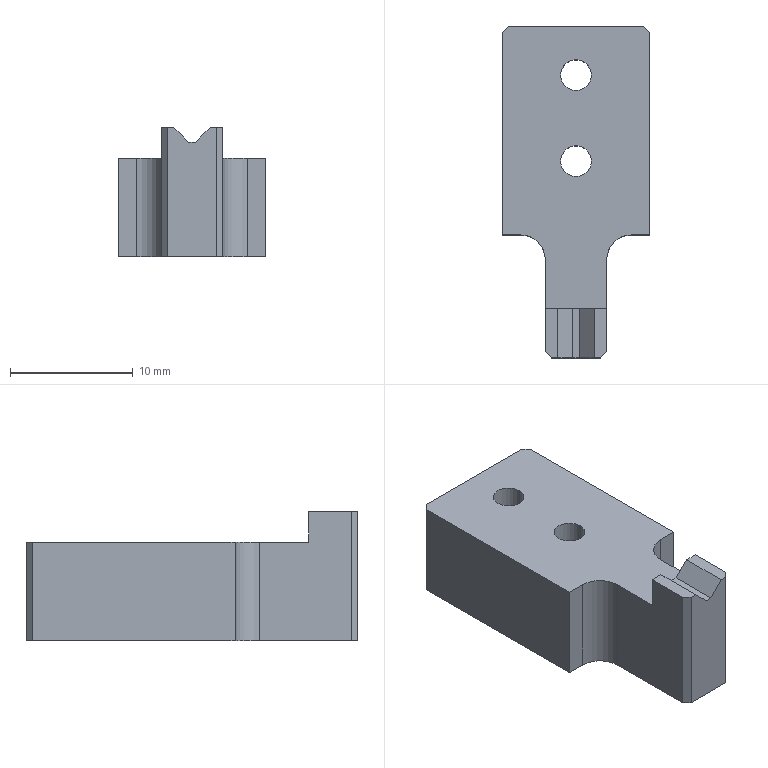Part | SolidWorks | features BaseBody 1 | 1 solid | 33 faces | box 12 x 27 x 10.5 mm | volume 1648 mm3 | plane 24 | cylinder 9 | commonest cylinder face diameters 2.5 x4 1 x3 4 x2
STEP:
#1=CARTESIAN_POINT('',(5.5,27.,-10.5));
#2=VERTEX_POINT('',#1);
#3=CARTESIAN_POINT('',(6.,26.5,-10.5));
#4=VERTEX_POINT('',#3);
#5=CARTESIAN_POINT('',(6.,26.5,-10.5));
#6=DIRECTION('',(0.7071,-0.7071,0.));
#7=VECTOR('',#6,1000.);
#8=LINE('',#5,#7);
#9=EDGE_CURVE('',#2,#4,#8,.T.);
#10=ORIENTED_EDGE('',*,*,#9,.F.);
#11=CARTESIAN_POINT('',(5.5,27.,-2.5));
#12=VERTEX_POINT('',#11);
#13=CARTESIAN_POINT('',(5.5,27.,-10.5));
#14=DIRECTION('',(0.,0.,-1.));
#15=VECTOR('',#14,1000.);
#16=LINE('',#13,#15);
#17=EDGE_CURVE('',#12,#2,#16,.T.);
#18=ORIENTED_EDGE('',*,*,#17,.F.);
#19=CARTESIAN_POINT('',(6.,26.5,-2.5));
#20=VERTEX_POINT('',#19);
#21=CARTESIAN_POINT('',(6.,26.5,-2.5));
#22=DIRECTION('',(-0.7071,0.7071,0.));
#23=VECTOR('',#22,1000.);
#24=LINE('',#21,#23);
#25=EDGE_CURVE('',#20,#12,#24,.T.);
#26=ORIENTED_EDGE('',*,*,#25,.F.);
#27=CARTESIAN_POINT('',(6.,26.5,-2.5));
#28=DIRECTION('',(0.,0.,1.));
#29=VECTOR('',#28,1000.);
#30=LINE('',#27,#29);
#31=EDGE_CURVE('',#4,#20,#30,.T.);
#32=ORIENTED_EDGE('',*,*,#31,.F.);
#33=EDGE_LOOP('',(#10,#18,#26,#32));
#34=FACE_OUTER_BOUND('',#33,.T.);
#35=CARTESIAN_POINT('',(6.,26.5,0.));
#36=DIRECTION('',(0.7071,0.7071,0.));
#37=DIRECTION('',(0.,0.,-1.));
#38=AXIS2_PLACEMENT_3D('',#35,#36,#37);
#39=PLANE('',#38);
#40=ADVANCED_FACE('',(#34),#39,.T.);
#41=CARTESIAN_POINT('',(-6.,26.5,-10.5));
#42=VERTEX_POINT('',#41);
#43=CARTESIAN_POINT('',(-5.5,27.,-10.5));
#44=VERTEX_POINT('',#43);
#45=CARTESIAN_POINT('',(-5.5,27.,-10.5));
#46=DIRECTION('',(0.7071,0.7071,0.));
#47=VECTOR('',#46,1000.);
#48=LINE('',#45,#47);
#49=EDGE_CURVE('',#42,#44,#48,.T.);
#50=ORIENTED_EDGE('',*,*,#49,.F.);
#51=CARTESIAN_POINT('',(-6.,26.5,-2.5));
#52=VERTEX_POINT('',#51);
#53=CARTESIAN_POINT('',(-6.,26.5,0.));
#54=DIRECTION('',(0.,0.,-1.));
#55=VECTOR('',#54,1000.);
#56=LINE('',#53,#55);
#57=EDGE_CURVE('',#52,#42,#56,.T.);
#58=ORIENTED_EDGE('',*,*,#57,.F.);
#59=CARTESIAN_POINT('',(-5.5,27.,-2.5));
#60=VERTEX_POINT('',#59);
#61=CARTESIAN_POINT('',(-5.5,27.,-2.5));
#62=DIRECTION('',(-0.7071,-0.7071,0.));
#63=VECTOR('',#62,1000.);
#64=LINE('',#61,#63);
#65=EDGE_CURVE('',#60,#52,#64,.T.);
#66=ORIENTED_EDGE('',*,*,#65,.F.);
#67=CARTESIAN_POINT('',(-5.5,27.,-2.5));
#68=DIRECTION('',(0.,0.,1.));
#69=VECTOR('',#68,1000.);
#70=LINE('',#67,#69);
#71=EDGE_CURVE('',#44,#60,#70,.T.);
#72=ORIENTED_EDGE('',*,*,#71,.F.);
#73=EDGE_LOOP('',(#50,#58,#66,#72));
#74=FACE_OUTER_BOUND('',#73,.T.);
#75=CARTESIAN_POINT('',(-5.5,27.,-2.5));
#76=DIRECTION('',(0.7071,-0.7071,0.));
#77=DIRECTION('',(0.,0.,-1.));
#78=AXIS2_PLACEMENT_3D('',#75,#76,#77);
#79=PLANE('',#78);
#80=ADVANCED_FACE('',(#74),#79,.F.);
#81=CARTESIAN_POINT('',(2.5,0.5,-10.5));
#82=VERTEX_POINT('',#81);
#83=CARTESIAN_POINT('',(2.,0.,-10.5));
#84=VERTEX_POINT('',#83);
#85=CARTESIAN_POINT('',(2.,0.,-10.5));
#86=DIRECTION('',(-0.7071,-0.7071,0.));
#87=VECTOR('',#86,1000.);
#88=LINE('',#85,#87);
#89=EDGE_CURVE('',#82,#84,#88,.T.);
#90=ORIENTED_EDGE('',*,*,#89,.F.);
#91=CARTESIAN_POINT('',(2.5,0.5,0.));
#92=VERTEX_POINT('',#91);
#93=CARTESIAN_POINT('',(2.5,0.5,-10.5));
#94=DIRECTION('',(0.,0.,-1.));
#95=VECTOR('',#94,1000.);
#96=LINE('',#93,#95);
#97=EDGE_CURVE('',#92,#82,#96,.T.);
#98=ORIENTED_EDGE('',*,*,#97,.F.);
#99=CARTESIAN_POINT('',(2.,0.,0.));
#100=VERTEX_POINT('',#99);
#101=CARTESIAN_POINT('',(2.,0.,0.));
#102=DIRECTION('',(0.7071,0.7071,0.));
#103=VECTOR('',#102,1000.);
#104=LINE('',#101,#103);
#105=EDGE_CURVE('',#100,#92,#104,.T.);
#106=ORIENTED_EDGE('',*,*,#105,.F.);
#107=CARTESIAN_POINT('',(2.,0.,-10.5));
#108=DIRECTION('',(0.,0.,1.));
#109=VECTOR('',#108,1000.);
#110=LINE('',#107,#109);
#111=EDGE_CURVE('',#84,#100,#110,.T.);
#112=ORIENTED_EDGE('',*,*,#111,.F.);
#113=EDGE_LOOP('',(#90,#98,#106,#112));
#114=FACE_OUTER_BOUND('',#113,.T.);
#115=CARTESIAN_POINT('',(2.,0.,-10.5));
#116=DIRECTION('',(-0.7071,0.7071,0.));
#117=DIRECTION('',(0.,0.,1.));
#118=AXIS2_PLACEMENT_3D('',#115,#116,#117);
#119=PLANE('',#118);
#120=ADVANCED_FACE('',(#114),#119,.F.);
#121=CARTESIAN_POINT('',(-2.,0.,-10.5));
#122=VERTEX_POINT('',#121);
#123=CARTESIAN_POINT('',(-2.5,0.5,-10.5));
#124=VERTEX_POINT('',#123);
#125=CARTESIAN_POINT('',(-2.5,0.5,-10.5));
#126=DIRECTION('',(-0.7071,0.7071,0.));
#127=VECTOR('',#126,1000.);
#128=LINE('',#125,#127);
#129=EDGE_CURVE('',#122,#124,#128,.T.);
#130=ORIENTED_EDGE('',*,*,#129,.F.);
#131=CARTESIAN_POINT('',(-2.,0.,0.));
#132=VERTEX_POINT('',#131);
#133=CARTESIAN_POINT('',(-2.,0.,-10.5));
#134=DIRECTION('',(0.,0.,-1.));
#135=VECTOR('',#134,1000.);
#136=LINE('',#133,#135);
#137=EDGE_CURVE('',#132,#122,#136,.T.);
#138=ORIENTED_EDGE('',*,*,#137,.F.);
#139=CARTESIAN_POINT('',(-2.5,0.5,0.));
#140=VERTEX_POINT('',#139);
#141=CARTESIAN_POINT('',(-2.5,0.5,0.));
#142=DIRECTION('',(0.7071,-0.7071,0.));
#143=VECTOR('',#142,1000.);
#144=LINE('',#141,#143);
#145=EDGE_CURVE('',#140,#132,#144,.T.);
#146=ORIENTED_EDGE('',*,*,#145,.F.);
#147=CARTESIAN_POINT('',(-2.5,0.5,-10.5));
#148=DIRECTION('',(0.,0.,1.));
#149=VECTOR('',#148,1000.);
#150=LINE('',#147,#149);
#151=EDGE_CURVE('',#124,#140,#150,.T.);
#152=ORIENTED_EDGE('',*,*,#151,.F.);
#153=EDGE_LOOP('',(#130,#138,#146,#152));
#154=FACE_OUTER_BOUND('',#153,.T.);
#155=CARTESIAN_POINT('',(-2.5,0.5,-10.5));
#156=DIRECTION('',(0.7071,0.7071,0.));
#157=DIRECTION('',(0.,0.,-1.));
#158=AXIS2_PLACEMENT_3D('',#155,#156,#157);
#159=PLANE('',#158);
#160=ADVANCED_FACE('',(#154),#159,.F.);
#161=CARTESIAN_POINT('',(4.5,10.,-10.5));
#162=VERTEX_POINT('',#161);
#163=CARTESIAN_POINT('',(4.5,10.,-2.5));
#164=VERTEX_POINT('',#163);
#165=CARTESIAN_POINT('',(4.5,10.,-10.5));
#166=DIRECTION('',(0.,0.,1.));
#167=VECTOR('',#166,1000.);
#168=LINE('',#165,#167);
#169=EDGE_CURVE('',#162,#164,#168,.T.);
#170=ORIENTED_EDGE('',*,*,#169,.F.);
#171=CARTESIAN_POINT('',(6.,10.,-10.5));
#172=VERTEX_POINT('',#171);
#173=CARTESIAN_POINT('',(6.,10.,-10.5));
#174=DIRECTION('',(-1.,0.,0.));
#175=VECTOR('',#174,1000.);
#176=LINE('',#173,#175);
#177=EDGE_CURVE('',#172,#162,#176,.T.);
#178=ORIENTED_EDGE('',*,*,#177,.F.);
#179=CARTESIAN_POINT('',(6.,10.,-2.5));
#180=VERTEX_POINT('',#179);
#181=CARTESIAN_POINT('',(6.,10.,-10.5));
#182=DIRECTION('',(0.,0.,1.));
#183=VECTOR('',#182,1000.);
#184=LINE('',#181,#183);
#185=EDGE_CURVE('',#172,#180,#184,.T.);
#186=ORIENTED_EDGE('',*,*,#185,.T.);
#187=CARTESIAN_POINT('',(6.,10.,-2.5));
#188=DIRECTION('',(1.,0.,0.));
#189=VECTOR('',#188,1000.);
#190=LINE('',#187,#189);
#191=EDGE_CURVE('',#164,#180,#190,.T.);
#192=ORIENTED_EDGE('',*,*,#191,.F.);
#193=EDGE_LOOP('',(#170,#178,#186,#192));
#194=FACE_OUTER_BOUND('',#193,.T.);
#195=CARTESIAN_POINT('',(6.,10.,-10.5));
#196=DIRECTION('',(0.,1.,0.));
#197=DIRECTION('',(1.,0.,0.));
#198=AXIS2_PLACEMENT_3D('',#195,#196,#197);
#199=PLANE('',#198);
#200=ADVANCED_FACE('',(#194),#199,.F.);
#201=CARTESIAN_POINT('',(2.5,8.,-10.5));
#202=VERTEX_POINT('',#201);
#203=CARTESIAN_POINT('',(2.5,8.,-2.5));
#204=VERTEX_POINT('',#203);
#205=CARTESIAN_POINT('',(2.5,8.,-10.5));
#206=DIRECTION('',(0.,0.,1.));
#207=VECTOR('',#206,1000.);
#208=LINE('',#205,#207);
#209=EDGE_CURVE('',#202,#204,#208,.T.);
#210=ORIENTED_EDGE('',*,*,#209,.F.);
#211=CARTESIAN_POINT('',(4.5,8.,-10.5));
#212=DIRECTION('',(0.,0.,1.));
#213=DIRECTION('',(1.,0.,0.));
#214=AXIS2_PLACEMENT_3D('',#211,#212,#213);
#215=CIRCLE('',#214,2.);
#216=EDGE_CURVE('',#162,#202,#215,.T.);
#217=ORIENTED_EDGE('',*,*,#216,.F.);
#218=ORIENTED_EDGE('',*,*,#169,.T.);
#219=CARTESIAN_POINT('',(4.5,8.,-2.5));
#220=DIRECTION('',(0.,0.,-1.));
#221=DIRECTION('',(-1.,0.,0.));
#222=AXIS2_PLACEMENT_3D('',#219,#220,#221);
#223=CIRCLE('',#222,2.);
#224=EDGE_CURVE('',#204,#164,#223,.T.);
#225=ORIENTED_EDGE('',*,*,#224,.F.);
#226=EDGE_LOOP('',(#210,#217,#218,#225));
#227=FACE_OUTER_BOUND('',#226,.T.);
#228=CARTESIAN_POINT('',(4.5,8.,-10.5));
#229=DIRECTION('',(0.,0.,1.));
#230=DIRECTION('',(1.,0.,0.));
#231=AXIS2_PLACEMENT_3D('',#228,#229,#230);
#232=CYLINDRICAL_SURFACE('',#231,2.);
#233=ADVANCED_FACE('',(#227),#232,.F.);
#234=CARTESIAN_POINT('',(2.5,4.,0.));
#235=VERTEX_POINT('',#234);
#236=CARTESIAN_POINT('',(2.5,0.,0.));
#237=DIRECTION('',(0.,-1.,0.));
#238=VECTOR('',#237,1000.);
#239=LINE('',#236,#238);
#240=EDGE_CURVE('',#235,#92,#239,.T.);
#241=ORIENTED_EDGE('',*,*,#240,.T.);
#242=ORIENTED_EDGE('',*,*,#97,.T.);
#243=CARTESIAN_POINT('',(2.5,0.,-10.5));
#244=DIRECTION('',(0.,-1.,0.));
#245=VECTOR('',#244,1000.);
#246=LINE('',#243,#245);
#247=EDGE_CURVE('',#202,#82,#246,.T.);
#248=ORIENTED_EDGE('',*,*,#247,.F.);
#249=ORIENTED_EDGE('',*,*,#209,.T.);
#250=CARTESIAN_POINT('',(2.5,4.,-2.5));
#251=VERTEX_POINT('',#250);
#252=CARTESIAN_POINT('',(2.5,4.,-2.5));
#253=DIRECTION('',(0.,1.,0.));
#254=VECTOR('',#253,1000.);
#255=LINE('',#252,#254);
#256=EDGE_CURVE('',#251,#204,#255,.T.);
#257=ORIENTED_EDGE('',*,*,#256,.F.);
#258=CARTESIAN_POINT('',(2.5,4.,-2.5));
#259=DIRECTION('',(0.,0.,-1.));
#260=VECTOR('',#259,1000.);
#261=LINE('',#258,#260);
#262=EDGE_CURVE('',#235,#251,#261,.T.);
#263=ORIENTED_EDGE('',*,*,#262,.F.);
#264=EDGE_LOOP('',(#241,#242,#248,#249,#257,#263));
#265=FACE_OUTER_BOUND('',#264,.T.);
#266=CARTESIAN_POINT('',(2.5,0.,-10.5));
#267=DIRECTION('',(-1.,0.,0.));
#268=DIRECTION('',(0.,1.,0.));
#269=AXIS2_PLACEMENT_3D('',#266,#267,#268);
#270=PLANE('',#269);
#271=ADVANCED_FACE('',(#265),#270,.F.);
#272=CARTESIAN_POINT('',(-6.,10.,-10.5));
#273=VERTEX_POINT('',#272);
#274=CARTESIAN_POINT('',(-6.,10.,-2.5));
#275=VERTEX_POINT('',#274);
#276=CARTESIAN_POINT('',(-6.,10.,-10.5));
#277=DIRECTION('',(0.,0.,1.));
#278=VECTOR('',#277,1000.);
#279=LINE('',#276,#278);
#280=EDGE_CURVE('',#273,#275,#279,.T.);
#281=ORIENTED_EDGE('',*,*,#280,.F.);
#282=CARTESIAN_POINT('',(-4.5,10.,-10.5));
#283=VERTEX_POINT('',#282);
#284=CARTESIAN_POINT('',(-6.,10.,-10.5));
#285=DIRECTION('',(-1.,0.,0.));
#286=VECTOR('',#285,1000.);
#287=LINE('',#284,#286);
#288=EDGE_CURVE('',#283,#273,#287,.T.);
#289=ORIENTED_EDGE('',*,*,#288,.F.);
#290=CARTESIAN_POINT('',(-4.5,10.,-2.5));
#291=VERTEX_POINT('',#290);
#292=CARTESIAN_POINT('',(-4.5,10.,-10.5));
#293=DIRECTION('',(0.,0.,1.));
#294=VECTOR('',#293,1000.);
#295=LINE('',#292,#294);
#296=EDGE_CURVE('',#283,#291,#295,.T.);
#297=ORIENTED_EDGE('',*,*,#296,.T.);
#298=CARTESIAN_POINT('',(6.,10.,-2.5));
#299=DIRECTION('',(1.,0.,0.));
#300=VECTOR('',#299,1000.);
#301=LINE('',#298,#300);
#302=EDGE_CURVE('',#275,#291,#301,.T.);
#303=ORIENTED_EDGE('',*,*,#302,.F.);
#304=EDGE_LOOP('',(#281,#289,#297,#303));
#305=FACE_OUTER_BOUND('',#304,.T.);
#306=CARTESIAN_POINT('',(-6.,10.,-10.5));
#307=DIRECTION('',(0.,1.,0.));
#308=DIRECTION('',(1.,0.,0.));
#309=AXIS2_PLACEMENT_3D('',#306,#307,#308);
#310=PLANE('',#309);
#311=ADVANCED_FACE('',(#305),#310,.F.);
#312=CARTESIAN_POINT('',(-2.5,8.,-10.5));
#313=VERTEX_POINT('',#312);
#314=CARTESIAN_POINT('',(-2.5,0.,-10.5));
#315=DIRECTION('',(0.,1.,0.));
#316=VECTOR('',#315,1000.);
#317=LINE('',#314,#316);
#318=EDGE_CURVE('',#124,#313,#317,.T.);
#319=ORIENTED_EDGE('',*,*,#318,.F.);
#320=ORIENTED_EDGE('',*,*,#151,.T.);
#321=CARTESIAN_POINT('',(-2.5,4.,0.));
#322=VERTEX_POINT('',#321);
#323=CARTESIAN_POINT('',(-2.5,0.,0.));
#324=DIRECTION('',(0.,1.,0.));
#325=VECTOR('',#324,1000.);
#326=LINE('',#323,#325);
#327=EDGE_CURVE('',#140,#322,#326,.T.);
#328=ORIENTED_EDGE('',*,*,#327,.T.);
#329=CARTESIAN_POINT('',(-2.5,4.,-2.5));
#330=VERTEX_POINT('',#329);
#331=CARTESIAN_POINT('',(-2.5,4.,-2.5));
#332=DIRECTION('',(0.,0.,1.));
#333=VECTOR('',#332,1000.);
#334=LINE('',#331,#333);
#335=EDGE_CURVE('',#330,#322,#334,.T.);
#336=ORIENTED_EDGE('',*,*,#335,.F.);
#337=CARTESIAN_POINT('',(-2.5,8.,-2.5));
#338=VERTEX_POINT('',#337);
#339=CARTESIAN_POINT('',(-2.5,4.,-2.5));
#340=DIRECTION('',(0.,-1.,0.));
#341=VECTOR('',#340,1000.);
#342=LINE('',#339,#341);
#343=EDGE_CURVE('',#338,#330,#342,.T.);
#344=ORIENTED_EDGE('',*,*,#343,.F.);
#345=CARTESIAN_POINT('',(-2.5,8.,-10.5));
#346=DIRECTION('',(0.,0.,1.));
#347=VECTOR('',#346,1000.);
#348=LINE('',#345,#347);
#349=EDGE_CURVE('',#313,#338,#348,.T.);
#350=ORIENTED_EDGE('',*,*,#349,.F.);
#351=EDGE_LOOP('',(#319,#320,#328,#336,#344,#350));
#352=FACE_OUTER_BOUND('',#351,.T.);
#353=CARTESIAN_POINT('',(-2.5,0.,-10.5));
#354=DIRECTION('',(1.,0.,0.));
#355=DIRECTION('',(0.,1.,0.));
#356=AXIS2_PLACEMENT_3D('',#353,#354,#355);
#357=PLANE('',#356);
#358=ADVANCED_FACE('',(#352),#357,.F.);
#359=ORIENTED_EDGE('',*,*,#296,.F.);
#360=CARTESIAN_POINT('',(-4.5,8.,-10.5));
#361=DIRECTION('',(0.,0.,1.));
#362=DIRECTION('',(1.,0.,0.));
#363=AXIS2_PLACEMENT_3D('',#360,#361,#362);
#364=CIRCLE('',#363,2.);
#365=EDGE_CURVE('',#313,#283,#364,.T.);
#366=ORIENTED_EDGE('',*,*,#365,.F.);
#367=ORIENTED_EDGE('',*,*,#349,.T.);
#368=CARTESIAN_POINT('',(-4.5,8.,-2.5));
#369=DIRECTION('',(0.,0.,-1.));
#370=DIRECTION('',(-1.,0.,0.));
#371=AXIS2_PLACEMENT_3D('',#368,#369,#370);
#372=CIRCLE('',#371,2.);
#373=EDGE_CURVE('',#291,#338,#372,.T.);
#374=ORIENTED_EDGE('',*,*,#373,.F.);
#375=EDGE_LOOP('',(#359,#366,#367,#374));
#376=FACE_OUTER_BOUND('',#375,.T.);
#377=CARTESIAN_POINT('',(-4.5,8.,-10.5));
#378=DIRECTION('',(0.,0.,1.));
#379=DIRECTION('',(1.,0.,0.));
#380=AXIS2_PLACEMENT_3D('',#377,#378,#379);
#381=CYLINDRICAL_SURFACE('',#380,2.);
#382=ADVANCED_FACE('',(#376),#381,.F.);
#383=CARTESIAN_POINT('',(-0.2799,4.,-1.2));
#384=VERTEX_POINT('',#383);
#385=CARTESIAN_POINT('',(-1.48,4.,0.));
#386=VERTEX_POINT('',#385);
#387=CARTESIAN_POINT('',(-1.48,4.,0.));
#388=DIRECTION('',(-0.7071,0.,0.7071));
#389=VECTOR('',#388,1000.);
#390=LINE('',#387,#389);
#391=EDGE_CURVE('',#384,#386,#390,.T.);
#392=ORIENTED_EDGE('',*,*,#391,.T.);
#393=CARTESIAN_POINT('',(-1.48,0.,0.));
#394=VERTEX_POINT('',#393);
#395=CARTESIAN_POINT('',(-1.48,27.001,0.));
#396=DIRECTION('',(0.,-1.,0.));
#397=VECTOR('',#396,1000.);
#398=LINE('',#395,#397);
#399=EDGE_CURVE('',#386,#394,#398,.T.);
#400=ORIENTED_EDGE('',*,*,#399,.T.);
#401=CARTESIAN_POINT('',(-0.2799,0.,-1.2));
#402=VERTEX_POINT('',#401);
#403=CARTESIAN_POINT('',(-1.48,0.,0.));
#404=DIRECTION('',(0.7071,0.,-0.7071));
#405=VECTOR('',#404,1000.);
#406=LINE('',#403,#405);
#407=EDGE_CURVE('',#394,#402,#406,.T.);
#408=ORIENTED_EDGE('',*,*,#407,.T.);
#409=CARTESIAN_POINT('',(-0.2799,27.001,-1.2));
#410=DIRECTION('',(0.,-1.,0.));
#411=VECTOR('',#410,1000.);
#412=LINE('',#409,#411);
#413=EDGE_CURVE('',#384,#402,#412,.T.);
#414=ORIENTED_EDGE('',*,*,#413,.F.);
#415=EDGE_LOOP('',(#392,#400,#408,#414));
#416=FACE_OUTER_BOUND('',#415,.T.);
#417=CARTESIAN_POINT('',(-1.48,27.001,0.));
#418=DIRECTION('',(-0.7071,0.,-0.7071));
#419=DIRECTION('',(-0.7071,0.,0.7071));
#420=AXIS2_PLACEMENT_3D('',#417,#418,#419);
#421=PLANE('',#420);
#422=ADVANCED_FACE('',(#416),#421,.F.);
#423=CARTESIAN_POINT('',(0.2799,4.,-1.2));
#424=VERTEX_POINT('',#423);
#425=CARTESIAN_POINT('',(-0.2799,4.,-1.2));
#426=DIRECTION('',(-1.,0.,0.));
#427=VECTOR('',#426,1000.);
#428=LINE('',#425,#427);
#429=EDGE_CURVE('',#424,#384,#428,.T.);
#430=ORIENTED_EDGE('',*,*,#429,.T.);
#431=ORIENTED_EDGE('',*,*,#413,.T.);
#432=CARTESIAN_POINT('',(0.2799,0.,-1.2));
#433=VERTEX_POINT('',#432);
#434=CARTESIAN_POINT('',(-0.2799,0.,-1.2));
#435=DIRECTION('',(1.,0.,0.));
#436=VECTOR('',#435,1000.);
#437=LINE('',#434,#436);
#438=EDGE_CURVE('',#402,#433,#437,.T.);
#439=ORIENTED_EDGE('',*,*,#438,.T.);
#440=CARTESIAN_POINT('',(0.2799,27.001,-1.2));
#441=DIRECTION('',(0.,-1.,0.));
#442=VECTOR('',#441,1000.);
#443=LINE('',#440,#442);
#444=EDGE_CURVE('',#424,#433,#443,.T.);
#445=ORIENTED_EDGE('',*,*,#444,.F.);
#446=EDGE_LOOP('',(#430,#431,#439,#445));
#447=FACE_OUTER_BOUND('',#446,.T.);
#448=CARTESIAN_POINT('',(-0.2799,27.001,-1.2));
#449=DIRECTION('',(0.,0.,-1.));
#450=DIRECTION('',(0.,-1.,0.));
#451=AXIS2_PLACEMENT_3D('',#448,#449,#450);
#452=PLANE('',#451);
#453=ADVANCED_FACE('',(#447),#452,.F.);
#454=CARTESIAN_POINT('',(1.48,4.,0.));
#455=VERTEX_POINT('',#454);
#456=CARTESIAN_POINT('',(0.2799,4.,-1.2));
#457=DIRECTION('',(-0.7071,0.,-0.7071));
#458=VECTOR('',#457,1000.);
#459=LINE('',#456,#458);
#460=EDGE_CURVE('',#455,#424,#459,.T.);
#461=ORIENTED_EDGE('',*,*,#460,.T.);
#462=ORIENTED_EDGE('',*,*,#444,.T.);
#463=CARTESIAN_POINT('',(1.48,0.,0.));
#464=VERTEX_POINT('',#463);
#465=CARTESIAN_POINT('',(0.2799,0.,-1.2));
#466=DIRECTION('',(0.7071,0.,0.7071));
#467=VECTOR('',#466,1000.);
#468=LINE('',#465,#467);
#469=EDGE_CURVE('',#433,#464,#468,.T.);
#470=ORIENTED_EDGE('',*,*,#469,.T.);
#471=CARTESIAN_POINT('',(1.48,27.001,0.));
#472=DIRECTION('',(0.,-1.,0.));
#473=VECTOR('',#472,1000.);
#474=LINE('',#471,#473);
#475=EDGE_CURVE('',#455,#464,#474,.T.);
#476=ORIENTED_EDGE('',*,*,#475,.F.);
#477=EDGE_LOOP('',(#461,#462,#470,#476));
#478=FACE_OUTER_BOUND('',#477,.T.);
#479=CARTESIAN_POINT('',(0.2799,27.001,-1.2));
#480=DIRECTION('',(0.7071,0.,-0.7071));
#481=DIRECTION('',(0.,-1.,0.));
#482=AXIS2_PLACEMENT_3D('',#479,#480,#481);
#483=PLANE('',#482);
#484=ADVANCED_FACE('',(#478),#483,.F.);
#485=CARTESIAN_POINT('',(1.25,23.,-2.5));
#486=VERTEX_POINT('',#485);
#487=CARTESIAN_POINT('',(1.25,23.,-7.3));
#488=VERTEX_POINT('',#487);
#489=CARTESIAN_POINT('',(1.25,23.,-7.3));
#490=DIRECTION('',(0.,0.,-1.));
#491=VECTOR('',#490,1000.);
#492=LINE('',#489,#491);
#493=EDGE_CURVE('',#486,#488,#492,.T.);
#494=ORIENTED_EDGE('',*,*,#493,.F.);
#495=CARTESIAN_POINT('',(-1.25,23.,-2.5));
#496=VERTEX_POINT('',#495);
#497=CARTESIAN_POINT('',(0.,23.,-2.5));
#498=DIRECTION('',(0.,0.,-1.));
#499=DIRECTION('',(-1.,0.,0.));
#500=AXIS2_PLACEMENT_3D('',#497,#498,#499);
#501=CIRCLE('',#500,1.25);
#502=EDGE_CURVE('',#496,#486,#501,.T.);
#503=ORIENTED_EDGE('',*,*,#502,.F.);
#504=CARTESIAN_POINT('',(-1.25,23.,-7.3));
#505=VERTEX_POINT('',#504);
#506=CARTESIAN_POINT('',(-1.25,23.,-7.3));
#507=DIRECTION('',(0.,0.,-1.));
#508=VECTOR('',#507,1000.);
#509=LINE('',#506,#508);
#510=EDGE_CURVE('',#496,#505,#509,.T.);
#511=ORIENTED_EDGE('',*,*,#510,.T.);
#512=CARTESIAN_POINT('',(0.,23.,-7.3));
#513=DIRECTION('',(0.,0.,-1.));
#514=DIRECTION('',(-1.,0.,0.));
#515=AXIS2_PLACEMENT_3D('',#512,#513,#514);
#516=CIRCLE('',#515,1.25);
#517=EDGE_CURVE('',#505,#488,#516,.T.);
#518=ORIENTED_EDGE('',*,*,#517,.T.);
#519=EDGE_LOOP('',(#494,#503,#511,#518));
#520=FACE_OUTER_BOUND('',#519,.T.);
#521=CARTESIAN_POINT('',(0.,23.,-7.3));
#522=DIRECTION('',(0.,0.,-1.));
#523=DIRECTION('',(-1.,0.,0.));
#524=AXIS2_PLACEMENT_3D('',#521,#522,#523);
#525=CYLINDRICAL_SURFACE('',#524,1.25);
#526=ADVANCED_FACE('',(#520),#525,.F.);
#527=CARTESIAN_POINT('',(1.25,16.,-2.5));
#528=VERTEX_POINT('',#527);
#529=CARTESIAN_POINT('',(1.25,16.,-7.3));
#530=VERTEX_POINT('',#529);
#531=CARTESIAN_POINT('',(1.25,16.,-7.3));
#532=DIRECTION('',(0.,0.,-1.));
#533=VECTOR('',#532,1000.);
#534=LINE('',#531,#533);
#535=EDGE_CURVE('',#528,#530,#534,.T.);
#536=ORIENTED_EDGE('',*,*,#535,.F.);
#537=CARTESIAN_POINT('',(-1.25,16.,-2.5));
#538=VERTEX_POINT('',#537);
#539=CARTESIAN_POINT('',(0.,16.,-2.5));
#540=DIRECTION('',(0.,0.,-1.));
#541=DIRECTION('',(-1.,0.,0.));
#542=AXIS2_PLACEMENT_3D('',#539,#540,#541);
#543=CIRCLE('',#542,1.25);
#544=EDGE_CURVE('',#538,#528,#543,.T.);
#545=ORIENTED_EDGE('',*,*,#544,.F.);
#546=CARTESIAN_POINT('',(-1.25,16.,-7.3));
#547=VERTEX_POINT('',#546);
#548=CARTESIAN_POINT('',(-1.25,16.,-7.3));
#549=DIRECTION('',(0.,0.,-1.));
#550=VECTOR('',#549,1000.);
#551=LINE('',#548,#550);
#552=EDGE_CURVE('',#538,#547,#551,.T.);
#553=ORIENTED_EDGE('',*,*,#552,.T.);
#554=CARTESIAN_POINT('',(0.,16.,-7.3));
#555=DIRECTION('',(0.,0.,-1.));
#556=DIRECTION('',(-1.,0.,0.));
#557=AXIS2_PLACEMENT_3D('',#554,#555,#556);
#558=CIRCLE('',#557,1.25);
#559=EDGE_CURVE('',#547,#530,#558,.T.);
#560=ORIENTED_EDGE('',*,*,#559,.T.);
#561=EDGE_LOOP('',(#536,#545,#553,#560));
#562=FACE_OUTER_BOUND('',#561,.T.);
#563=CARTESIAN_POINT('',(0.,16.,-7.3));
#564=DIRECTION('',(0.,0.,-1.));
#565=DIRECTION('',(-1.,0.,0.));
#566=AXIS2_PLACEMENT_3D('',#563,#564,#565);
#567=CYLINDRICAL_SURFACE('',#566,1.25);
#568=ADVANCED_FACE('',(#562),#567,.F.);
#569=ORIENTED_EDGE('',*,*,#559,.F.);
#570=CARTESIAN_POINT('',(0.,16.,-7.3));
#571=DIRECTION('',(0.,0.,-1.));
#572=DIRECTION('',(-1.,0.,0.));
#573=AXIS2_PLACEMENT_3D('',#570,#571,#572);
#574=CIRCLE('',#573,1.25);
#575=EDGE_CURVE('',#530,#547,#574,.T.);
#576=ORIENTED_EDGE('',*,*,#575,.F.);
#577=EDGE_LOOP('',(#569,#576));
#578=FACE_BOUND('',#577,.T.);
#579=ORIENTED_EDGE('',*,*,#517,.F.);
#580=CARTESIAN_POINT('',(0.,23.,-7.3));
#581=DIRECTION('',(0.,0.,-1.));
#582=DIRECTION('',(-1.,0.,0.));
#583=AXIS2_PLACEMENT_3D('',#580,#581,#582);
#584=CIRCLE('',#583,1.25);
#585=EDGE_CURVE('',#488,#505,#584,.T.);
#586=ORIENTED_EDGE('',*,*,#585,.F.);
#587=EDGE_LOOP('',(#579,#586));
#588=FACE_BOUND('',#587,.T.);
#589=CARTESIAN_POINT('',(-4.,27.,-7.3));
#590=VERTEX_POINT('',#589);
#591=CARTESIAN_POINT('',(-4.,12.5,-7.3));
#592=VERTEX_POINT('',#591);
#593=CARTESIAN_POINT('',(-4.,27.,-7.3));
#594=DIRECTION('',(0.,-1.,0.));
#595=VECTOR('',#594,1000.);
#596=LINE('',#593,#595);
#597=EDGE_CURVE('',#590,#592,#596,.T.);
#598=ORIENTED_EDGE('',*,*,#597,.F.);
#599=CARTESIAN_POINT('',(4.,27.,-7.3));
#600=VERTEX_POINT('',#599);
#601=CARTESIAN_POINT('',(-4.,27.,-7.3));
#602=DIRECTION('',(-1.,0.,0.));
#603=VECTOR('',#602,1000.);
#604=LINE('',#601,#603);
#605=EDGE_CURVE('',#600,#590,#604,.T.);
#606=ORIENTED_EDGE('',*,*,#605,.F.);
#607=CARTESIAN_POINT('',(4.,12.5,-7.3));
#608=VERTEX_POINT('',#607);
#609=CARTESIAN_POINT('',(4.,27.,-7.3));
#610=DIRECTION('',(0.,1.,0.));
#611=VECTOR('',#610,1000.);
#612=LINE('',#609,#611);
#613=EDGE_CURVE('',#608,#600,#612,.T.);
#614=ORIENTED_EDGE('',*,*,#613,.F.);
#615=CARTESIAN_POINT('',(3.5,12.,-7.3));
#616=VERTEX_POINT('',#615);
#617=CARTESIAN_POINT('',(4.,12.,-7.3));
#618=DIRECTION('',(0.,0.,1.));
#619=DIRECTION('',(1.,0.,0.));
#620=AXIS2_PLACEMENT_3D('',#617,#618,#619);
#621=CIRCLE('',#620,0.5);
#622=EDGE_CURVE('',#616,#608,#621,.T.);
#623=ORIENTED_EDGE('',*,*,#622,.F.);
#624=CARTESIAN_POINT('',(-3.5,12.,-7.3));
#625=VERTEX_POINT('',#624);
#626=CARTESIAN_POINT('',(-3.5,12.,-7.3));
#627=DIRECTION('',(1.,0.,0.));
#628=VECTOR('',#627,1000.);
#629=LINE('',#626,#628);
#630=EDGE_CURVE('',#625,#616,#629,.T.);
#631=ORIENTED_EDGE('',*,*,#630,.F.);
#632=CARTESIAN_POINT('',(-4.5,12.,-7.3));
#633=VERTEX_POINT('',#632);
#634=CARTESIAN_POINT('',(-4.,12.,-7.3));
#635=DIRECTION('',(0.,0.,1.));
#636=DIRECTION('',(1.,0.,0.));
#637=AXIS2_PLACEMENT_3D('',#634,#635,#636);
#638=CIRCLE('',#637,0.5);
#639=EDGE_CURVE('',#633,#625,#638,.T.);
#640=ORIENTED_EDGE('',*,*,#639,.F.);
#641=CARTESIAN_POINT('',(-4.,12.,-7.3));
#642=DIRECTION('',(0.,0.,1.));
#643=DIRECTION('',(1.,0.,0.));
#644=AXIS2_PLACEMENT_3D('',#641,#642,#643);
#645=CIRCLE('',#644,0.5);
#646=EDGE_CURVE('',#592,#633,#645,.T.);
#647=ORIENTED_EDGE('',*,*,#646,.F.);
#648=EDGE_LOOP('',(#598,#606,#614,#623,#631,#640,#647));
#649=FACE_OUTER_BOUND('',#648,.T.);
#650=CARTESIAN_POINT('',(-4.,12.,-7.3));
#651=DIRECTION('',(0.,0.,1.));
#652=DIRECTION('',(1.,0.,0.));
#653=AXIS2_PLACEMENT_3D('',#650,#651,#652);
#654=PLANE('',#653);
#655=ADVANCED_FACE('',(#578,#588,#649),#654,.F.);
#656=CARTESIAN_POINT('',(4.,12.5,-10.5));
#657=VERTEX_POINT('',#656);
#658=CARTESIAN_POINT('',(4.,27.,-10.5));
#659=VERTEX_POINT('',#658);
#660=CARTESIAN_POINT('',(4.,27.,-10.5));
#661=DIRECTION('',(0.,1.,0.));
#662=VECTOR('',#661,1000.);
#663=LINE('',#660,#662);
#664=EDGE_CURVE('',#657,#659,#663,.T.);
#665=ORIENTED_EDGE('',*,*,#664,.F.);
#666=CARTESIAN_POINT('',(4.,12.5,-7.3));
#667=DIRECTION('',(0.,0.,-1.));
#668=VECTOR('',#667,1000.);
#669=LINE('',#666,#668);
#670=EDGE_CURVE('',#608,#657,#669,.T.);
#671=ORIENTED_EDGE('',*,*,#670,.F.);
#672=ORIENTED_EDGE('',*,*,#613,.T.);
#673=CARTESIAN_POINT('',(4.,27.,-7.3));
#674=DIRECTION('',(0.,0.,-1.));
#675=VECTOR('',#674,1000.);
#676=LINE('',#673,#675);
#677=EDGE_CURVE('',#600,#659,#676,.T.);
#678=ORIENTED_EDGE('',*,*,#677,.T.);
#679=EDGE_LOOP('',(#665,#671,#672,#678));
#680=FACE_OUTER_BOUND('',#679,.T.);
#681=CARTESIAN_POINT('',(4.,27.,-7.3));
#682=DIRECTION('',(-1.,0.,0.));
#683=DIRECTION('',(0.,1.,0.));
#684=AXIS2_PLACEMENT_3D('',#681,#682,#683);
#685=PLANE('',#684);
#686=ADVANCED_FACE('',(#680),#685,.T.);
#687=CARTESIAN_POINT('',(3.5,12.,-10.5));
#688=VERTEX_POINT('',#687);
#689=CARTESIAN_POINT('',(4.,12.,-10.5));
#690=DIRECTION('',(0.,0.,1.));
#691=DIRECTION('',(1.,0.,0.));
#692=AXIS2_PLACEMENT_3D('',#689,#690,#691);
#693=CIRCLE('',#692,0.5);
#694=EDGE_CURVE('',#688,#657,#693,.T.);
#695=ORIENTED_EDGE('',*,*,#694,.F.);
#696=CARTESIAN_POINT('',(3.5,12.,-7.3));
#697=DIRECTION('',(0.,0.,-1.));
#698=VECTOR('',#697,1000.);
#699=LINE('',#696,#698);
#700=EDGE_CURVE('',#616,#688,#699,.T.);
#701=ORIENTED_EDGE('',*,*,#700,.F.);
#702=ORIENTED_EDGE('',*,*,#622,.T.);
#703=ORIENTED_EDGE('',*,*,#670,.T.);
#704=EDGE_LOOP('',(#695,#701,#702,#703));
#705=FACE_OUTER_BOUND('',#704,.T.);
#706=CARTESIAN_POINT('',(4.,12.,-7.3));
#707=DIRECTION('',(0.,0.,-1.));
#708=DIRECTION('',(-1.,0.,0.));
#709=AXIS2_PLACEMENT_3D('',#706,#707,#708);
#710=CYLINDRICAL_SURFACE('',#709,0.5);
#711=ADVANCED_FACE('',(#705),#710,.F.);
#712=CARTESIAN_POINT('',(-3.5,12.,-10.5));
#713=VERTEX_POINT('',#712);
#714=CARTESIAN_POINT('',(-3.5,12.,-10.5));
#715=DIRECTION('',(1.,0.,0.));
#716=VECTOR('',#715,1000.);
#717=LINE('',#714,#716);
#718=EDGE_CURVE('',#713,#688,#717,.T.);
#719=ORIENTED_EDGE('',*,*,#718,.F.);
#720=CARTESIAN_POINT('',(-3.5,12.,-7.3));
#721=DIRECTION('',(0.,0.,-1.));
#722=VECTOR('',#721,1000.);
#723=LINE('',#720,#722);
#724=EDGE_CURVE('',#625,#713,#723,.T.);
#725=ORIENTED_EDGE('',*,*,#724,.F.);
#726=ORIENTED_EDGE('',*,*,#630,.T.);
#727=ORIENTED_EDGE('',*,*,#700,.T.);
#728=EDGE_LOOP('',(#719,#725,#726,#727));
#729=FACE_OUTER_BOUND('',#728,.T.);
#730=CARTESIAN_POINT('',(-3.5,12.,-7.3));
#731=DIRECTION('',(0.,1.,0.));
#732=DIRECTION('',(1.,0.,0.));
#733=AXIS2_PLACEMENT_3D('',#730,#731,#732);
#734=PLANE('',#733);
#735=ADVANCED_FACE('',(#729),#734,.T.);
#736=CARTESIAN_POINT('',(-4.5,12.,-10.5));
#737=VERTEX_POINT('',#736);
#738=CARTESIAN_POINT('',(-4.5,12.,-7.3));
#739=DIRECTION('',(0.,0.,-1.));
#740=VECTOR('',#739,1000.);
#741=LINE('',#738,#740);
#742=EDGE_CURVE('',#633,#737,#741,.T.);
#743=ORIENTED_EDGE('',*,*,#742,.F.);
#744=ORIENTED_EDGE('',*,*,#639,.T.);
#745=ORIENTED_EDGE('',*,*,#724,.T.);
#746=CARTESIAN_POINT('',(-4.,12.,-10.5));
#747=DIRECTION('',(0.,0.,1.));
#748=DIRECTION('',(1.,0.,0.));
#749=AXIS2_PLACEMENT_3D('',#746,#747,#748);
#750=CIRCLE('',#749,0.5);
#751=EDGE_CURVE('',#737,#713,#750,.T.);
#752=ORIENTED_EDGE('',*,*,#751,.F.);
#753=EDGE_LOOP('',(#743,#744,#745,#752));
#754=FACE_OUTER_BOUND('',#753,.T.);
#755=CARTESIAN_POINT('',(-4.,12.,-7.3));
#756=DIRECTION('',(0.,0.,-1.));
#757=DIRECTION('',(-1.,0.,0.));
#758=AXIS2_PLACEMENT_3D('',#755,#756,#757);
#759=CYLINDRICAL_SURFACE('',#758,0.5);
#760=ADVANCED_FACE('',(#754),#759,.F.);
#761=CARTESIAN_POINT('',(-4.,27.,-10.5));
#762=VERTEX_POINT('',#761);
#763=CARTESIAN_POINT('',(-4.,12.5,-10.5));
#764=VERTEX_POINT('',#763);
#765=CARTESIAN_POINT('',(-4.,27.,-10.5));
#766=DIRECTION('',(0.,-1.,0.));
#767=VECTOR('',#766,1000.);
#768=LINE('',#765,#767);
#769=EDGE_CURVE('',#762,#764,#768,.T.);
#770=ORIENTED_EDGE('',*,*,#769,.F.);
#771=CARTESIAN_POINT('',(-4.,27.,-7.3));
#772=DIRECTION('',(0.,0.,-1.));
#773=VECTOR('',#772,1000.);
#774=LINE('',#771,#773);
#775=EDGE_CURVE('',#590,#762,#774,.T.);
#776=ORIENTED_EDGE('',*,*,#775,.F.);
#777=ORIENTED_EDGE('',*,*,#597,.T.);
#778=CARTESIAN_POINT('',(-4.,12.5,-7.3));
#779=DIRECTION('',(0.,0.,-1.));
#780=VECTOR('',#779,1000.);
#781=LINE('',#778,#780);
#782=EDGE_CURVE('',#592,#764,#781,.T.);
#783=ORIENTED_EDGE('',*,*,#782,.T.);
#784=EDGE_LOOP('',(#770,#776,#777,#783));
#785=FACE_OUTER_BOUND('',#784,.T.);
#786=CARTESIAN_POINT('',(-4.,27.,-7.3));
#787=DIRECTION('',(1.,0.,0.));
#788=DIRECTION('',(0.,1.,0.));
#789=AXIS2_PLACEMENT_3D('',#786,#787,#788);
#790=PLANE('',#789);
#791=ADVANCED_FACE('',(#785),#790,.T.);
#792=CARTESIAN_POINT('',(-6.,4.,-2.5));
#793=DIRECTION('',(0.,-1.,0.));
#794=VECTOR('',#793,1000.);
#795=LINE('',#792,#794);
#796=EDGE_CURVE('',#52,#275,#795,.T.);
#797=ORIENTED_EDGE('',*,*,#796,.F.);
#798=ORIENTED_EDGE('',*,*,#57,.T.);
#799=CARTESIAN_POINT('',(-6.,27.,-10.5));
#800=DIRECTION('',(0.,1.,0.));
#801=VECTOR('',#800,1000.);
#802=LINE('',#799,#801);
#803=EDGE_CURVE('',#273,#42,#802,.T.);
#804=ORIENTED_EDGE('',*,*,#803,.F.);
#805=ORIENTED_EDGE('',*,*,#280,.T.);
#806=EDGE_LOOP('',(#797,#798,#804,#805));
#807=FACE_OUTER_BOUND('',#806,.T.);
#808=CARTESIAN_POINT('',(-6.,0.,0.));
#809=DIRECTION('',(1.,0.,0.));
#810=DIRECTION('',(0.,1.,0.));
#811=AXIS2_PLACEMENT_3D('',#808,#809,#810);
#812=PLANE('',#811);
#813=ADVANCED_FACE('',(#807),#812,.F.);
#814=CARTESIAN_POINT('',(6.,27.,-10.5));
#815=DIRECTION('',(0.,1.,0.));
#816=VECTOR('',#815,1000.);
#817=LINE('',#814,#816);
#818=EDGE_CURVE('',#172,#4,#817,.T.);
#819=ORIENTED_EDGE('',*,*,#818,.T.);
#820=ORIENTED_EDGE('',*,*,#31,.T.);
#821=CARTESIAN_POINT('',(6.,4.,-2.5));
#822=DIRECTION('',(0.,-1.,0.));
#823=VECTOR('',#822,1000.);
#824=LINE('',#821,#823);
#825=EDGE_CURVE('',#20,#180,#824,.T.);
#826=ORIENTED_EDGE('',*,*,#825,.T.);
#827=ORIENTED_EDGE('',*,*,#185,.F.);
#828=EDGE_LOOP('',(#819,#820,#826,#827));
#829=FACE_OUTER_BOUND('',#828,.T.);
#830=CARTESIAN_POINT('',(6.,0.,0.));
#831=DIRECTION('',(1.,0.,0.));
#832=DIRECTION('',(0.,1.,0.));
#833=AXIS2_PLACEMENT_3D('',#830,#831,#832);
#834=PLANE('',#833);
#835=ADVANCED_FACE('',(#829),#834,.T.);
#836=ORIENTED_EDGE('',*,*,#544,.T.);
#837=CARTESIAN_POINT('',(0.,16.,-2.5));
#838=DIRECTION('',(0.,0.,-1.));
#839=DIRECTION('',(-1.,0.,0.));
#840=AXIS2_PLACEMENT_3D('',#837,#838,#839);
#841=CIRCLE('',#840,1.25);
#842=EDGE_CURVE('',#528,#538,#841,.T.);
#843=ORIENTED_EDGE('',*,*,#842,.T.);
#844=EDGE_LOOP('',(#836,#843));
#845=FACE_BOUND('',#844,.T.);
#846=ORIENTED_EDGE('',*,*,#502,.T.);
#847=CARTESIAN_POINT('',(0.,23.,-2.5));
#848=DIRECTION('',(0.,0.,-1.));
#849=DIRECTION('',(-1.,0.,0.));
#850=AXIS2_PLACEMENT_3D('',#847,#848,#849);
#851=CIRCLE('',#850,1.25);
#852=EDGE_CURVE('',#486,#496,#851,.T.);
#853=ORIENTED_EDGE('',*,*,#852,.T.);
#854=EDGE_LOOP('',(#846,#853));
#855=FACE_BOUND('',#854,.T.);
#856=CARTESIAN_POINT('',(6.,27.,-2.5));
#857=DIRECTION('',(-1.,0.,0.));
#858=VECTOR('',#857,1000.);
#859=LINE('',#856,#858);
#860=EDGE_CURVE('',#12,#60,#859,.T.);
#861=ORIENTED_EDGE('',*,*,#860,.T.);
#862=ORIENTED_EDGE('',*,*,#65,.T.);
#863=ORIENTED_EDGE('',*,*,#796,.T.);
#864=ORIENTED_EDGE('',*,*,#302,.T.);
#865=ORIENTED_EDGE('',*,*,#373,.T.);
#866=ORIENTED_EDGE('',*,*,#343,.T.);
#867=CARTESIAN_POINT('',(6.,4.,-2.5));
#868=DIRECTION('',(-1.,0.,0.));
#869=VECTOR('',#868,1000.);
#870=LINE('',#867,#869);
#871=EDGE_CURVE('',#251,#330,#870,.T.);
#872=ORIENTED_EDGE('',*,*,#871,.F.);
#873=ORIENTED_EDGE('',*,*,#256,.T.);
#874=ORIENTED_EDGE('',*,*,#224,.T.);
#875=ORIENTED_EDGE('',*,*,#191,.T.);
#876=ORIENTED_EDGE('',*,*,#825,.F.);
#877=ORIENTED_EDGE('',*,*,#25,.T.);
#878=EDGE_LOOP('',(#861,#862,#863,#864,#865,#866,#872,#873,#874,#875,#876,#877));
#879=FACE_OUTER_BOUND('',#878,.T.);
#880=CARTESIAN_POINT('',(6.,4.,-2.5));
#881=DIRECTION('',(0.,0.,-1.));
#882=DIRECTION('',(0.,-1.,0.));
#883=AXIS2_PLACEMENT_3D('',#880,#881,#882);
#884=PLANE('',#883);
#885=ADVANCED_FACE('',(#845,#855,#879),#884,.F.);
#886=CARTESIAN_POINT('',(6.,0.,0.));
#887=DIRECTION('',(-1.,0.,0.));
#888=VECTOR('',#887,1000.);
#889=LINE('',#886,#888);
#890=EDGE_CURVE('',#394,#132,#889,.T.);
#891=ORIENTED_EDGE('',*,*,#890,.T.);
#892=ORIENTED_EDGE('',*,*,#137,.T.);
#893=CARTESIAN_POINT('',(6.,0.,-10.5));
#894=DIRECTION('',(-1.,0.,0.));
#895=VECTOR('',#894,1000.);
#896=LINE('',#893,#895);
#897=EDGE_CURVE('',#84,#122,#896,.T.);
#898=ORIENTED_EDGE('',*,*,#897,.F.);
#899=ORIENTED_EDGE('',*,*,#111,.T.);
#900=CARTESIAN_POINT('',(6.,0.,0.));
#901=DIRECTION('',(-1.,0.,0.));
#902=VECTOR('',#901,1000.);
#903=LINE('',#900,#902);
#904=EDGE_CURVE('',#100,#464,#903,.T.);
#905=ORIENTED_EDGE('',*,*,#904,.T.);
#906=ORIENTED_EDGE('',*,*,#469,.F.);
#907=ORIENTED_EDGE('',*,*,#438,.F.);
#908=ORIENTED_EDGE('',*,*,#407,.F.);
#909=EDGE_LOOP('',(#891,#892,#898,#899,#905,#906,#907,#908));
#910=FACE_OUTER_BOUND('',#909,.T.);
#911=CARTESIAN_POINT('',(6.,0.,-10.5));
#912=DIRECTION('',(0.,1.,0.));
#913=DIRECTION('',(0.,0.,-1.));
#914=AXIS2_PLACEMENT_3D('',#911,#912,#913);
#915=PLANE('',#914);
#916=ADVANCED_FACE('',(#910),#915,.F.);
#917=ORIENTED_EDGE('',*,*,#327,.F.);
#918=ORIENTED_EDGE('',*,*,#145,.T.);
#919=ORIENTED_EDGE('',*,*,#890,.F.);
#920=ORIENTED_EDGE('',*,*,#399,.F.);
#921=CARTESIAN_POINT('',(6.,4.,0.));
#922=DIRECTION('',(-1.,0.,0.));
#923=VECTOR('',#922,1000.);
#924=LINE('',#921,#923);
#925=EDGE_CURVE('',#386,#322,#924,.T.);
#926=ORIENTED_EDGE('',*,*,#925,.T.);
#927=EDGE_LOOP('',(#917,#918,#919,#920,#926));
#928=FACE_OUTER_BOUND('',#927,.T.);
#929=CARTESIAN_POINT('',(6.,4.,0.));
#930=DIRECTION('',(0.,0.,-1.));
#931=DIRECTION('',(0.,-1.,0.));
#932=AXIS2_PLACEMENT_3D('',#929,#930,#931);
#933=PLANE('',#932);
#934=ADVANCED_FACE('',(#928),#933,.F.);
#935=CARTESIAN_POINT('',(6.,4.,0.));
#936=DIRECTION('',(-1.,0.,0.));
#937=VECTOR('',#936,1000.);
#938=LINE('',#935,#937);
#939=EDGE_CURVE('',#235,#455,#938,.T.);
#940=ORIENTED_EDGE('',*,*,#939,.F.);
#941=ORIENTED_EDGE('',*,*,#262,.T.);
#942=ORIENTED_EDGE('',*,*,#871,.T.);
#943=ORIENTED_EDGE('',*,*,#335,.T.);
#944=ORIENTED_EDGE('',*,*,#925,.F.);
#945=ORIENTED_EDGE('',*,*,#391,.F.);
#946=ORIENTED_EDGE('',*,*,#429,.F.);
#947=ORIENTED_EDGE('',*,*,#460,.F.);
#948=EDGE_LOOP('',(#940,#941,#942,#943,#944,#945,#946,#947));
#949=FACE_OUTER_BOUND('',#948,.T.);
#950=CARTESIAN_POINT('',(6.,4.,-2.5));
#951=DIRECTION('',(0.,-1.,0.));
#952=DIRECTION('',(0.,0.,-1.));
#953=AXIS2_PLACEMENT_3D('',#950,#951,#952);
#954=PLANE('',#953);
#955=ADVANCED_FACE('',(#949),#954,.F.);
#956=CARTESIAN_POINT('',(6.,27.,-10.5));
#957=DIRECTION('',(-1.,0.,0.));
#958=VECTOR('',#957,1000.);
#959=LINE('',#956,#958);
#960=EDGE_CURVE('',#762,#44,#959,.T.);
#961=ORIENTED_EDGE('',*,*,#960,.T.);
#962=ORIENTED_EDGE('',*,*,#71,.T.);
#963=ORIENTED_EDGE('',*,*,#860,.F.);
#964=ORIENTED_EDGE('',*,*,#17,.T.);
#965=CARTESIAN_POINT('',(6.,27.,-10.5));
#966=DIRECTION('',(-1.,0.,0.));
#967=VECTOR('',#966,1000.);
#968=LINE('',#965,#967);
#969=EDGE_CURVE('',#2,#659,#968,.T.);
#970=ORIENTED_EDGE('',*,*,#969,.T.);
#971=ORIENTED_EDGE('',*,*,#677,.F.);
#972=ORIENTED_EDGE('',*,*,#605,.T.);
#973=ORIENTED_EDGE('',*,*,#775,.T.);
#974=EDGE_LOOP('',(#961,#962,#963,#964,#970,#971,#972,#973));
#975=FACE_OUTER_BOUND('',#974,.T.);
#976=CARTESIAN_POINT('',(6.,27.,-2.5));
#977=DIRECTION('',(0.,-1.,0.));
#978=DIRECTION('',(0.,0.,-1.));
#979=AXIS2_PLACEMENT_3D('',#976,#977,#978);
#980=PLANE('',#979);
#981=ADVANCED_FACE('',(#975),#980,.F.);
#982=ORIENTED_EDGE('',*,*,#897,.T.);
#983=ORIENTED_EDGE('',*,*,#129,.T.);
#984=ORIENTED_EDGE('',*,*,#318,.T.);
#985=ORIENTED_EDGE('',*,*,#365,.T.);
#986=ORIENTED_EDGE('',*,*,#288,.T.);
#987=ORIENTED_EDGE('',*,*,#803,.T.);
#988=ORIENTED_EDGE('',*,*,#49,.T.);
#989=ORIENTED_EDGE('',*,*,#960,.F.);
#990=ORIENTED_EDGE('',*,*,#769,.T.);
#991=CARTESIAN_POINT('',(-4.,12.,-10.5));
#992=DIRECTION('',(0.,0.,1.));
#993=DIRECTION('',(1.,0.,0.));
#994=AXIS2_PLACEMENT_3D('',#991,#992,#993);
#995=CIRCLE('',#994,0.5);
#996=EDGE_CURVE('',#764,#737,#995,.T.);
#997=ORIENTED_EDGE('',*,*,#996,.T.);
#998=ORIENTED_EDGE('',*,*,#751,.T.);
#999=ORIENTED_EDGE('',*,*,#718,.T.);
#1000=ORIENTED_EDGE('',*,*,#694,.T.);
#1001=ORIENTED_EDGE('',*,*,#664,.T.);
#1002=ORIENTED_EDGE('',*,*,#969,.F.);
#1003=ORIENTED_EDGE('',*,*,#9,.T.);
#1004=ORIENTED_EDGE('',*,*,#818,.F.);
#1005=ORIENTED_EDGE('',*,*,#177,.T.);
#1006=ORIENTED_EDGE('',*,*,#216,.T.);
#1007=ORIENTED_EDGE('',*,*,#247,.T.);
#1008=ORIENTED_EDGE('',*,*,#89,.T.);
#1009=EDGE_LOOP('',(#982,#983,#984,#985,#986,#987,#988,#989,#990,#997,#998,#999,#1000,#1001,#1002,#1003,#1004,#1005,#1006,#1007,#1008));
#1010=FACE_OUTER_BOUND('',#1009,.T.);
#1011=CARTESIAN_POINT('',(6.,27.,-10.5));
#1012=DIRECTION('',(0.,0.,1.));
#1013=DIRECTION('',(0.,-1.,0.));
#1014=AXIS2_PLACEMENT_3D('',#1011,#1012,#1013);
#1015=PLANE('',#1014);
#1016=ADVANCED_FACE('',(#1010),#1015,.F.);
#1017=ORIENTED_EDGE('',*,*,#904,.F.);
#1018=ORIENTED_EDGE('',*,*,#105,.T.);
#1019=ORIENTED_EDGE('',*,*,#240,.F.);
#1020=ORIENTED_EDGE('',*,*,#939,.T.);
#1021=ORIENTED_EDGE('',*,*,#475,.T.);
#1022=EDGE_LOOP('',(#1017,#1018,#1019,#1020,#1021));
#1023=FACE_OUTER_BOUND('',#1022,.T.);
#1024=CARTESIAN_POINT('',(6.,4.,0.));
#1025=DIRECTION('',(0.,0.,-1.));
#1026=DIRECTION('',(0.,-1.,0.));
#1027=AXIS2_PLACEMENT_3D('',#1024,#1025,#1026);
#1028=PLANE('',#1027);
#1029=ADVANCED_FACE('',(#1023),#1028,.F.);
#1030=ORIENTED_EDGE('',*,*,#646,.T.);
#1031=ORIENTED_EDGE('',*,*,#742,.T.);
#1032=ORIENTED_EDGE('',*,*,#996,.F.);
#1033=ORIENTED_EDGE('',*,*,#782,.F.);
#1034=EDGE_LOOP('',(#1030,#1031,#1032,#1033));
#1035=FACE_OUTER_BOUND('',#1034,.T.);
#1036=CARTESIAN_POINT('',(-4.,12.,-7.3));
#1037=DIRECTION('',(0.,0.,-1.));
#1038=DIRECTION('',(-1.,0.,0.));
#1039=AXIS2_PLACEMENT_3D('',#1036,#1037,#1038);
#1040=CYLINDRICAL_SURFACE('',#1039,0.5);
#1041=ADVANCED_FACE('',(#1035),#1040,.F.);
#1042=ORIENTED_EDGE('',*,*,#842,.F.);
#1043=ORIENTED_EDGE('',*,*,#535,.T.);
#1044=ORIENTED_EDGE('',*,*,#575,.T.);
#1045=ORIENTED_EDGE('',*,*,#552,.F.);
#1046=EDGE_LOOP('',(#1042,#1043,#1044,#1045));
#1047=FACE_OUTER_BOUND('',#1046,.T.);
#1048=CARTESIAN_POINT('',(0.,16.,-7.3));
#1049=DIRECTION('',(0.,0.,-1.));
#1050=DIRECTION('',(-1.,0.,0.));
#1051=AXIS2_PLACEMENT_3D('',#1048,#1049,#1050);
#1052=CYLINDRICAL_SURFACE('',#1051,1.25);
#1053=ADVANCED_FACE('',(#1047),#1052,.F.);
#1054=ORIENTED_EDGE('',*,*,#852,.F.);
#1055=ORIENTED_EDGE('',*,*,#493,.T.);
#1056=ORIENTED_EDGE('',*,*,#585,.T.);
#1057=ORIENTED_EDGE('',*,*,#510,.F.);
#1058=EDGE_LOOP('',(#1054,#1055,#1056,#1057));
#1059=FACE_OUTER_BOUND('',#1058,.T.);
#1060=CARTESIAN_POINT('',(0.,23.,-7.3));
#1061=DIRECTION('',(0.,0.,-1.));
#1062=DIRECTION('',(-1.,0.,0.));
#1063=AXIS2_PLACEMENT_3D('',#1060,#1061,#1062);
#1064=CYLINDRICAL_SURFACE('',#1063,1.25);
#1065=ADVANCED_FACE('',(#1059),#1064,.F.);
#1066=CLOSED_SHELL('',(#40,#80,#120,#160,#200,#233,#271,#311,#358,#382,#422,#453,#484,#526,#568,#655,#686,#711,#735,#760,#791,#813,#835,#885,#916,#934,#955,#981,#1016,#1029,#1041,#1053,#1065));
#1067=MANIFOLD_SOLID_BREP('',#1066);
#1068=CARTESIAN_POINT('',(0.,0.,0.));
#1069=DIRECTION('',(0.,0.,1.));
#1070=DIRECTION('',(1.,0.,0.));
#1071=AXIS2_PLACEMENT_3D('',#1068,#1069,#1070);
#1072=(LENGTH_UNIT()NAMED_UNIT(*)SI_UNIT(.MILLI.,.METRE.));
#1073=UNCERTAINTY_MEASURE_WITH_UNIT(LENGTH_MEASURE(0.00001),#1072,'','');
#1074=(NAMED_UNIT(*)PLANE_ANGLE_UNIT()SI_UNIT($,.RADIAN.));
#1075=(NAMED_UNIT(*)SI_UNIT($,.STERADIAN.)SOLID_ANGLE_UNIT());
#1076=(GEOMETRIC_REPRESENTATION_CONTEXT(3)GLOBAL_UNCERTAINTY_ASSIGNED_CONTEXT((#1073))GLOBAL_UNIT_ASSIGNED_CONTEXT((#1072,#1074,#1075))REPRESENTATION_CONTEXT('',''));
#1077=ADVANCED_BREP_SHAPE_REPRESENTATION('',(#1067,#1071),#1076);